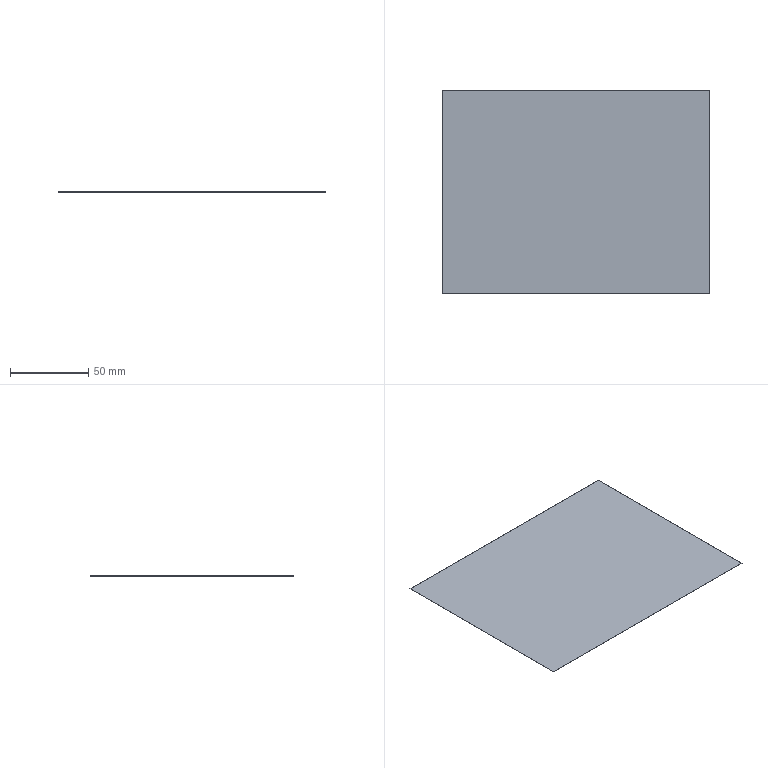Part | STEP file | [蔬沉] | 1 solid | 6 faces | box 170 x 130 x 0.1 mm | volume 2210 mm3 | plane 6
STEP:
#1=CARTESIAN_POINT('',(0.,0.,0.));
#2=DIRECTION('',(0.,0.,1.));
#3=DIRECTION('',(1.,0.,0.));
#4=AXIS2_PLACEMENT_3D('',#1,#2,#3);
#5=CARTESIAN_POINT('',(0.,130.,0.));
#6=VERTEX_POINT('',#5);
#7=CARTESIAN_POINT('',(170.,130.,0.));
#8=VERTEX_POINT('',#7);
#9=CARTESIAN_POINT('',(85.,130.,0.));
#10=DIRECTION('',(1.,0.,0.));
#11=VECTOR('',#10,1.);
#12=LINE('',#9,#11);
#13=CARTESIAN_POINT('',(85.,130.,0.05));
#14=DIRECTION('',(0.,1.,0.));
#15=DIRECTION('',(-1.,0.,0.));
#16=AXIS2_PLACEMENT_3D('',#13,#14,#15);
#17=PLANE('',#16);
#18=CARTESIAN_POINT('',(0.,-0.05));
#19=DIRECTION('',(-1.,0.));
#20=VECTOR('',#19,1.);
#21=LINE('',#18,#20);
#22=(GEOMETRIC_REPRESENTATION_CONTEXT(2)PARAMETRIC_REPRESENTATION_CONTEXT()REPRESENTATION_CONTEXT('',''));
#23=DEFINITIONAL_REPRESENTATION('',(#21),#22);
#24=PCURVE('',#17,#23);
#25=CARTESIAN_POINT('',(85.,0.,0.));
#26=DIRECTION('',(0.,0.,-1.));
#27=DIRECTION('',(0.,-1.,0.));
#28=AXIS2_PLACEMENT_3D('',#25,#26,#27);
#29=PLANE('',#28);
#30=CARTESIAN_POINT('',(-130.,0.));
#31=DIRECTION('',(0.,-1.));
#32=VECTOR('',#31,1.);
#33=LINE('',#30,#32);
#34=(GEOMETRIC_REPRESENTATION_CONTEXT(2)PARAMETRIC_REPRESENTATION_CONTEXT()REPRESENTATION_CONTEXT('',''));
#35=DEFINITIONAL_REPRESENTATION('',(#33),#34);
#36=PCURVE('',#29,#35);
#37=SURFACE_CURVE('',#12,(#24,#36),.PCURVE_S1.);
#38=EDGE_CURVE('',#6,#8,#37,.T.);
#39=ORIENTED_EDGE('',*,*,#38,.F.);
#40=CARTESIAN_POINT('',(0.,130.,0.1));
#41=VERTEX_POINT('',#40);
#42=CARTESIAN_POINT('',(0.,130.,0.05));
#43=DIRECTION('',(0.,0.,-1.));
#44=VECTOR('',#43,1.);
#45=LINE('',#42,#44);
#46=CARTESIAN_POINT('',(85.,0.));
#47=DIRECTION('',(0.,-1.));
#48=VECTOR('',#47,1.);
#49=LINE('',#46,#48);
#50=(GEOMETRIC_REPRESENTATION_CONTEXT(2)PARAMETRIC_REPRESENTATION_CONTEXT()REPRESENTATION_CONTEXT('',''));
#51=DEFINITIONAL_REPRESENTATION('',(#49),#50);
#52=PCURVE('',#17,#51);
#53=CARTESIAN_POINT('',(0.,0.,0.05));
#54=DIRECTION('',(-1.,0.,0.));
#55=DIRECTION('',(0.,-1.,0.));
#56=AXIS2_PLACEMENT_3D('',#53,#54,#55);
#57=PLANE('',#56);
#58=CARTESIAN_POINT('',(-130.,0.));
#59=DIRECTION('',(0.,-1.));
#60=VECTOR('',#59,1.);
#61=LINE('',#58,#60);
#62=(GEOMETRIC_REPRESENTATION_CONTEXT(2)PARAMETRIC_REPRESENTATION_CONTEXT()REPRESENTATION_CONTEXT('',''));
#63=DEFINITIONAL_REPRESENTATION('',(#61),#62);
#64=PCURVE('',#57,#63);
#65=SURFACE_CURVE('',#45,(#52,#64),.PCURVE_S1.);
#66=EDGE_CURVE('',#41,#6,#65,.T.);
#67=ORIENTED_EDGE('',*,*,#66,.F.);
#68=CARTESIAN_POINT('',(170.,130.,0.1));
#69=VERTEX_POINT('',#68);
#70=CARTESIAN_POINT('',(85.,130.,0.1));
#71=DIRECTION('',(-1.,0.,0.));
#72=VECTOR('',#71,1.);
#73=LINE('',#70,#72);
#74=CARTESIAN_POINT('',(0.,0.05));
#75=DIRECTION('',(1.,0.));
#76=VECTOR('',#75,1.);
#77=LINE('',#74,#76);
#78=(GEOMETRIC_REPRESENTATION_CONTEXT(2)PARAMETRIC_REPRESENTATION_CONTEXT()REPRESENTATION_CONTEXT('',''));
#79=DEFINITIONAL_REPRESENTATION('',(#77),#78);
#80=PCURVE('',#17,#79);
#81=CARTESIAN_POINT('',(85.,0.,0.1));
#82=DIRECTION('',(0.,0.,1.));
#83=DIRECTION('',(0.,1.,0.));
#84=AXIS2_PLACEMENT_3D('',#81,#82,#83);
#85=PLANE('',#84);
#86=CARTESIAN_POINT('',(130.,0.));
#87=DIRECTION('',(0.,1.));
#88=VECTOR('',#87,1.);
#89=LINE('',#86,#88);
#90=(GEOMETRIC_REPRESENTATION_CONTEXT(2)PARAMETRIC_REPRESENTATION_CONTEXT()REPRESENTATION_CONTEXT('',''));
#91=DEFINITIONAL_REPRESENTATION('',(#89),#90);
#92=PCURVE('',#85,#91);
#93=SURFACE_CURVE('',#73,(#80,#92),.PCURVE_S1.);
#94=EDGE_CURVE('',#69,#41,#93,.T.);
#95=ORIENTED_EDGE('',*,*,#94,.F.);
#96=CARTESIAN_POINT('',(170.,130.,0.05));
#97=DIRECTION('',(0.,0.,1.));
#98=VECTOR('',#97,1.);
#99=LINE('',#96,#98);
#100=CARTESIAN_POINT('',(-85.,0.));
#101=DIRECTION('',(0.,1.));
#102=VECTOR('',#101,1.);
#103=LINE('',#100,#102);
#104=(GEOMETRIC_REPRESENTATION_CONTEXT(2)PARAMETRIC_REPRESENTATION_CONTEXT()REPRESENTATION_CONTEXT('',''));
#105=DEFINITIONAL_REPRESENTATION('',(#103),#104);
#106=PCURVE('',#17,#105);
#107=CARTESIAN_POINT('',(170.,0.,0.05));
#108=DIRECTION('',(1.,0.,0.));
#109=DIRECTION('',(0.,1.,0.));
#110=AXIS2_PLACEMENT_3D('',#107,#108,#109);
#111=PLANE('',#110);
#112=CARTESIAN_POINT('',(130.,0.));
#113=DIRECTION('',(0.,1.));
#114=VECTOR('',#113,1.);
#115=LINE('',#112,#114);
#116=(GEOMETRIC_REPRESENTATION_CONTEXT(2)PARAMETRIC_REPRESENTATION_CONTEXT()REPRESENTATION_CONTEXT('',''));
#117=DEFINITIONAL_REPRESENTATION('',(#115),#116);
#118=PCURVE('',#111,#117);
#119=SURFACE_CURVE('',#99,(#106,#118),.PCURVE_S1.);
#120=EDGE_CURVE('',#8,#69,#119,.T.);
#121=ORIENTED_EDGE('',*,*,#120,.F.);
#122=EDGE_LOOP('',(#39,#67,#95,#121));
#123=FACE_BOUND('',#122,.T.);
#124=ADVANCED_FACE('',(#123),#17,.T.);
#125=CARTESIAN_POINT('',(0.,0.,0.));
#126=VERTEX_POINT('',#125);
#127=CARTESIAN_POINT('',(0.,0.,0.));
#128=DIRECTION('',(0.,1.,0.));
#129=VECTOR('',#128,1.);
#130=LINE('',#127,#129);
#131=CARTESIAN_POINT('',(0.,85.));
#132=DIRECTION('',(-1.,0.));
#133=VECTOR('',#132,1.);
#134=LINE('',#131,#133);
#135=(GEOMETRIC_REPRESENTATION_CONTEXT(2)PARAMETRIC_REPRESENTATION_CONTEXT()REPRESENTATION_CONTEXT('',''));
#136=DEFINITIONAL_REPRESENTATION('',(#134),#135);
#137=PCURVE('',#29,#136);
#138=CARTESIAN_POINT('',(0.,-0.05));
#139=DIRECTION('',(-1.,0.));
#140=VECTOR('',#139,1.);
#141=LINE('',#138,#140);
#142=(GEOMETRIC_REPRESENTATION_CONTEXT(2)PARAMETRIC_REPRESENTATION_CONTEXT()REPRESENTATION_CONTEXT('',''));
#143=DEFINITIONAL_REPRESENTATION('',(#141),#142);
#144=PCURVE('',#57,#143);
#145=SURFACE_CURVE('',#130,(#137,#144),.PCURVE_S1.);
#146=EDGE_CURVE('',#126,#6,#145,.T.);
#147=ORIENTED_EDGE('',*,*,#146,.T.);
#148=ORIENTED_EDGE('',*,*,#38,.T.);
#149=CARTESIAN_POINT('',(170.,0.,0.));
#150=VERTEX_POINT('',#149);
#151=CARTESIAN_POINT('',(170.,0.,0.));
#152=DIRECTION('',(0.,1.,0.));
#153=VECTOR('',#152,1.);
#154=LINE('',#151,#153);
#155=CARTESIAN_POINT('',(0.,-85.));
#156=DIRECTION('',(-1.,0.));
#157=VECTOR('',#156,1.);
#158=LINE('',#155,#157);
#159=(GEOMETRIC_REPRESENTATION_CONTEXT(2)PARAMETRIC_REPRESENTATION_CONTEXT()REPRESENTATION_CONTEXT('',''));
#160=DEFINITIONAL_REPRESENTATION('',(#158),#159);
#161=PCURVE('',#29,#160);
#162=CARTESIAN_POINT('',(0.,-0.05));
#163=DIRECTION('',(1.,0.));
#164=VECTOR('',#163,1.);
#165=LINE('',#162,#164);
#166=(GEOMETRIC_REPRESENTATION_CONTEXT(2)PARAMETRIC_REPRESENTATION_CONTEXT()REPRESENTATION_CONTEXT('',''));
#167=DEFINITIONAL_REPRESENTATION('',(#165),#166);
#168=PCURVE('',#111,#167);
#169=SURFACE_CURVE('',#154,(#161,#168),.PCURVE_S1.);
#170=EDGE_CURVE('',#150,#8,#169,.T.);
#171=ORIENTED_EDGE('',*,*,#170,.F.);
#172=CARTESIAN_POINT('',(85.,0.,0.));
#173=DIRECTION('',(-1.,0.,0.));
#174=VECTOR('',#173,1.);
#175=LINE('',#172,#174);
#176=CARTESIAN_POINT('',(0.,0.));
#177=DIRECTION('',(0.,1.));
#178=VECTOR('',#177,1.);
#179=LINE('',#176,#178);
#180=(GEOMETRIC_REPRESENTATION_CONTEXT(2)PARAMETRIC_REPRESENTATION_CONTEXT()REPRESENTATION_CONTEXT('',''));
#181=DEFINITIONAL_REPRESENTATION('',(#179),#180);
#182=PCURVE('',#29,#181);
#183=CARTESIAN_POINT('',(85.,0.,0.05));
#184=DIRECTION('',(0.,-1.,0.));
#185=DIRECTION('',(1.,0.,0.));
#186=AXIS2_PLACEMENT_3D('',#183,#184,#185);
#187=PLANE('',#186);
#188=CARTESIAN_POINT('',(0.,-0.05));
#189=DIRECTION('',(-1.,0.));
#190=VECTOR('',#189,1.);
#191=LINE('',#188,#190);
#192=(GEOMETRIC_REPRESENTATION_CONTEXT(2)PARAMETRIC_REPRESENTATION_CONTEXT()REPRESENTATION_CONTEXT('',''));
#193=DEFINITIONAL_REPRESENTATION('',(#191),#192);
#194=PCURVE('',#187,#193);
#195=SURFACE_CURVE('',#175,(#182,#194),.PCURVE_S1.);
#196=EDGE_CURVE('',#150,#126,#195,.T.);
#197=ORIENTED_EDGE('',*,*,#196,.T.);
#198=EDGE_LOOP('',(#147,#148,#171,#197));
#199=FACE_BOUND('',#198,.T.);
#200=ADVANCED_FACE('',(#199),#29,.T.);
#201=ORIENTED_EDGE('',*,*,#170,.T.);
#202=ORIENTED_EDGE('',*,*,#120,.T.);
#203=CARTESIAN_POINT('',(170.,0.,0.1));
#204=VERTEX_POINT('',#203);
#205=CARTESIAN_POINT('',(170.,0.,0.1));
#206=DIRECTION('',(0.,1.,0.));
#207=VECTOR('',#206,1.);
#208=LINE('',#205,#207);
#209=CARTESIAN_POINT('',(0.,0.05));
#210=DIRECTION('',(1.,0.));
#211=VECTOR('',#210,1.);
#212=LINE('',#209,#211);
#213=(GEOMETRIC_REPRESENTATION_CONTEXT(2)PARAMETRIC_REPRESENTATION_CONTEXT()REPRESENTATION_CONTEXT('',''));
#214=DEFINITIONAL_REPRESENTATION('',(#212),#213);
#215=PCURVE('',#111,#214);
#216=CARTESIAN_POINT('',(0.,-85.));
#217=DIRECTION('',(1.,0.));
#218=VECTOR('',#217,1.);
#219=LINE('',#216,#218);
#220=(GEOMETRIC_REPRESENTATION_CONTEXT(2)PARAMETRIC_REPRESENTATION_CONTEXT()REPRESENTATION_CONTEXT('',''));
#221=DEFINITIONAL_REPRESENTATION('',(#219),#220);
#222=PCURVE('',#85,#221);
#223=SURFACE_CURVE('',#208,(#215,#222),.PCURVE_S1.);
#224=EDGE_CURVE('',#204,#69,#223,.T.);
#225=ORIENTED_EDGE('',*,*,#224,.F.);
#226=CARTESIAN_POINT('',(170.,0.,0.05));
#227=DIRECTION('',(0.,0.,-1.));
#228=VECTOR('',#227,1.);
#229=LINE('',#226,#228);
#230=CARTESIAN_POINT('',(0.,0.));
#231=DIRECTION('',(0.,-1.));
#232=VECTOR('',#231,1.);
#233=LINE('',#230,#232);
#234=(GEOMETRIC_REPRESENTATION_CONTEXT(2)PARAMETRIC_REPRESENTATION_CONTEXT()REPRESENTATION_CONTEXT('',''));
#235=DEFINITIONAL_REPRESENTATION('',(#233),#234);
#236=PCURVE('',#111,#235);
#237=CARTESIAN_POINT('',(85.,0.));
#238=DIRECTION('',(0.,-1.));
#239=VECTOR('',#238,1.);
#240=LINE('',#237,#239);
#241=(GEOMETRIC_REPRESENTATION_CONTEXT(2)PARAMETRIC_REPRESENTATION_CONTEXT()REPRESENTATION_CONTEXT('',''));
#242=DEFINITIONAL_REPRESENTATION('',(#240),#241);
#243=PCURVE('',#187,#242);
#244=SURFACE_CURVE('',#229,(#236,#243),.PCURVE_S1.);
#245=EDGE_CURVE('',#204,#150,#244,.T.);
#246=ORIENTED_EDGE('',*,*,#245,.T.);
#247=EDGE_LOOP('',(#201,#202,#225,#246));
#248=FACE_BOUND('',#247,.T.);
#249=ADVANCED_FACE('',(#248),#111,.T.);
#250=ORIENTED_EDGE('',*,*,#224,.T.);
#251=ORIENTED_EDGE('',*,*,#94,.T.);
#252=CARTESIAN_POINT('',(0.,0.,0.1));
#253=VERTEX_POINT('',#252);
#254=CARTESIAN_POINT('',(0.,0.,0.1));
#255=DIRECTION('',(0.,1.,0.));
#256=VECTOR('',#255,1.);
#257=LINE('',#254,#256);
#258=CARTESIAN_POINT('',(0.,85.));
#259=DIRECTION('',(1.,0.));
#260=VECTOR('',#259,1.);
#261=LINE('',#258,#260);
#262=(GEOMETRIC_REPRESENTATION_CONTEXT(2)PARAMETRIC_REPRESENTATION_CONTEXT()REPRESENTATION_CONTEXT('',''));
#263=DEFINITIONAL_REPRESENTATION('',(#261),#262);
#264=PCURVE('',#85,#263);
#265=CARTESIAN_POINT('',(0.,0.05));
#266=DIRECTION('',(-1.,0.));
#267=VECTOR('',#266,1.);
#268=LINE('',#265,#267);
#269=(GEOMETRIC_REPRESENTATION_CONTEXT(2)PARAMETRIC_REPRESENTATION_CONTEXT()REPRESENTATION_CONTEXT('',''));
#270=DEFINITIONAL_REPRESENTATION('',(#268),#269);
#271=PCURVE('',#57,#270);
#272=SURFACE_CURVE('',#257,(#264,#271),.PCURVE_S1.);
#273=EDGE_CURVE('',#253,#41,#272,.T.);
#274=ORIENTED_EDGE('',*,*,#273,.F.);
#275=CARTESIAN_POINT('',(85.,0.,0.1));
#276=DIRECTION('',(1.,0.,0.));
#277=VECTOR('',#276,1.);
#278=LINE('',#275,#277);
#279=CARTESIAN_POINT('',(0.,0.));
#280=DIRECTION('',(0.,-1.));
#281=VECTOR('',#280,1.);
#282=LINE('',#279,#281);
#283=(GEOMETRIC_REPRESENTATION_CONTEXT(2)PARAMETRIC_REPRESENTATION_CONTEXT()REPRESENTATION_CONTEXT('',''));
#284=DEFINITIONAL_REPRESENTATION('',(#282),#283);
#285=PCURVE('',#85,#284);
#286=CARTESIAN_POINT('',(0.,0.05));
#287=DIRECTION('',(1.,0.));
#288=VECTOR('',#287,1.);
#289=LINE('',#286,#288);
#290=(GEOMETRIC_REPRESENTATION_CONTEXT(2)PARAMETRIC_REPRESENTATION_CONTEXT()REPRESENTATION_CONTEXT('',''));
#291=DEFINITIONAL_REPRESENTATION('',(#289),#290);
#292=PCURVE('',#187,#291);
#293=SURFACE_CURVE('',#278,(#285,#292),.PCURVE_S1.);
#294=EDGE_CURVE('',#253,#204,#293,.T.);
#295=ORIENTED_EDGE('',*,*,#294,.T.);
#296=EDGE_LOOP('',(#250,#251,#274,#295));
#297=FACE_BOUND('',#296,.T.);
#298=ADVANCED_FACE('',(#297),#85,.T.);
#299=CARTESIAN_POINT('',(0.,0.,0.05));
#300=DIRECTION('',(0.,0.,1.));
#301=VECTOR('',#300,1.);
#302=LINE('',#299,#301);
#303=CARTESIAN_POINT('',(-85.,0.));
#304=DIRECTION('',(0.,1.));
#305=VECTOR('',#304,1.);
#306=LINE('',#303,#305);
#307=(GEOMETRIC_REPRESENTATION_CONTEXT(2)PARAMETRIC_REPRESENTATION_CONTEXT()REPRESENTATION_CONTEXT('',''));
#308=DEFINITIONAL_REPRESENTATION('',(#306),#307);
#309=PCURVE('',#187,#308);
#310=CARTESIAN_POINT('',(0.,0.));
#311=DIRECTION('',(0.,1.));
#312=VECTOR('',#311,1.);
#313=LINE('',#310,#312);
#314=(GEOMETRIC_REPRESENTATION_CONTEXT(2)PARAMETRIC_REPRESENTATION_CONTEXT()REPRESENTATION_CONTEXT('',''));
#315=DEFINITIONAL_REPRESENTATION('',(#313),#314);
#316=PCURVE('',#57,#315);
#317=SURFACE_CURVE('',#302,(#309,#316),.PCURVE_S1.);
#318=EDGE_CURVE('',#126,#253,#317,.T.);
#319=ORIENTED_EDGE('',*,*,#318,.F.);
#320=ORIENTED_EDGE('',*,*,#196,.F.);
#321=ORIENTED_EDGE('',*,*,#245,.F.);
#322=ORIENTED_EDGE('',*,*,#294,.F.);
#323=EDGE_LOOP('',(#319,#320,#321,#322));
#324=FACE_BOUND('',#323,.T.);
#325=ADVANCED_FACE('',(#324),#187,.T.);
#326=ORIENTED_EDGE('',*,*,#318,.T.);
#327=ORIENTED_EDGE('',*,*,#273,.T.);
#328=ORIENTED_EDGE('',*,*,#66,.T.);
#329=ORIENTED_EDGE('',*,*,#146,.F.);
#330=EDGE_LOOP('',(#326,#327,#328,#329));
#331=FACE_BOUND('',#330,.T.);
#332=ADVANCED_FACE('',(#331),#57,.T.);
#333=CLOSED_SHELL('',(#124,#200,#249,#298,#325,#332));
#334=MANIFOLD_SOLID_BREP('',#333);
#335=(LENGTH_UNIT()NAMED_UNIT(*)SI_UNIT(.MILLI.,.METRE.));
#336=UNCERTAINTY_MEASURE_WITH_UNIT(LENGTH_MEASURE(0.0000001),#335,'','');
#337=(NAMED_UNIT(*)PLANE_ANGLE_UNIT()SI_UNIT($,.RADIAN.));
#338=(NAMED_UNIT(*)SI_UNIT($,.STERADIAN.)SOLID_ANGLE_UNIT());
#339=(GEOMETRIC_REPRESENTATION_CONTEXT(3)GLOBAL_UNCERTAINTY_ASSIGNED_CONTEXT((#336))GLOBAL_UNIT_ASSIGNED_CONTEXT((#335,#337,#338))REPRESENTATION_CONTEXT('',''));
#340=ADVANCED_BREP_SHAPE_REPRESENTATION('',(#4,#334),#339);